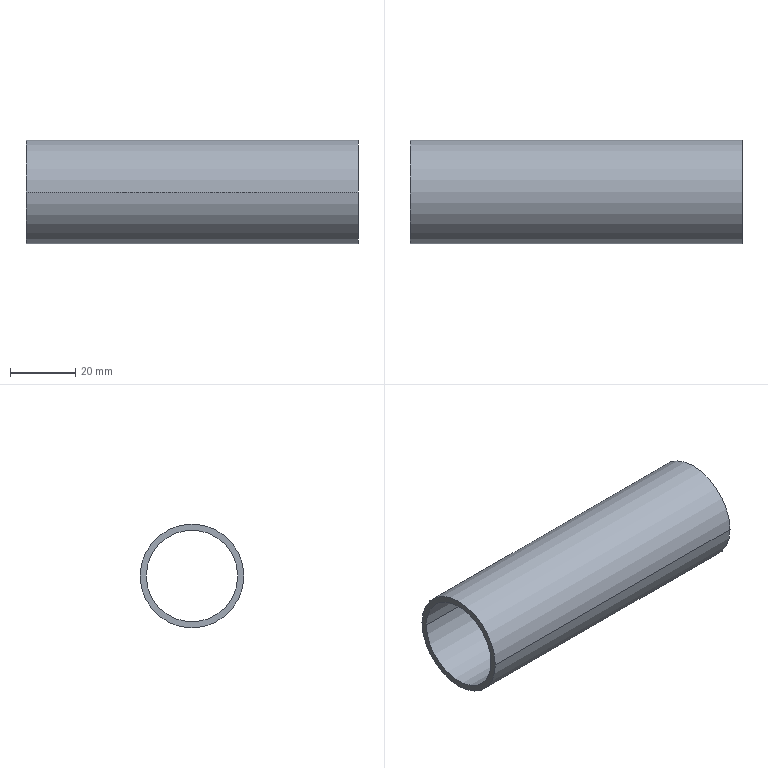Part | NX | features BREP 1 | 1 solid | 6 faces | box 101.6 x 31.75 x 31.75 mm | volume 17920 mm3 | cylinder 4 | plane 2 | commonest cylinder face diameters 27.991 x2 31.75 x2
STEP:
#1=CARTESIAN_POINT('',(0.,15.875,0.));
#2=VERTEX_POINT('',#1);
#3=CARTESIAN_POINT('',(0.,-15.875,0.));
#4=VERTEX_POINT('',#3);
#5=CARTESIAN_POINT('',(0.,0.,0.));
#6=DIRECTION('',(1.,0.,0.));
#7=DIRECTION('',(0.,1.,0.));
#8=AXIS2_PLACEMENT_3D('',#5,#6,#7);
#9=CIRCLE('',#8,15.875);
#10=EDGE_CURVE('',#2,#4,#9,.T.);
#11=ORIENTED_EDGE('',*,*,#10,.F.);
#12=CARTESIAN_POINT('',(0.,0.,0.));
#13=DIRECTION('',(1.,0.,0.));
#14=DIRECTION('',(0.,-1.,0.));
#15=AXIS2_PLACEMENT_3D('',#12,#13,#14);
#16=CIRCLE('',#15,15.875);
#17=EDGE_CURVE('',#4,#2,#16,.T.);
#18=ORIENTED_EDGE('',*,*,#17,.F.);
#19=EDGE_LOOP('',(#11,#18));
#20=FACE_BOUND('',#19,.T.);
#21=CARTESIAN_POINT('',(0.,13.995,0.));
#22=VERTEX_POINT('',#21);
#23=CARTESIAN_POINT('',(0.,-13.995,0.));
#24=VERTEX_POINT('',#23);
#25=CARTESIAN_POINT('',(0.,0.,0.));
#26=DIRECTION('',(-1.,0.,0.));
#27=DIRECTION('',(0.,1.,0.));
#28=AXIS2_PLACEMENT_3D('',#25,#26,#27);
#29=CIRCLE('',#28,13.995);
#30=EDGE_CURVE('',#22,#24,#29,.T.);
#31=ORIENTED_EDGE('',*,*,#30,.F.);
#32=CARTESIAN_POINT('',(0.,0.,0.));
#33=DIRECTION('',(-1.,0.,0.));
#34=DIRECTION('',(0.,-1.,0.));
#35=AXIS2_PLACEMENT_3D('',#32,#33,#34);
#36=CIRCLE('',#35,13.995);
#37=EDGE_CURVE('',#24,#22,#36,.T.);
#38=ORIENTED_EDGE('',*,*,#37,.F.);
#39=EDGE_LOOP('',(#31,#38));
#40=FACE_BOUND('',#39,.T.);
#41=CARTESIAN_POINT('',(0.,0.,0.));
#42=DIRECTION('',(1.,0.,0.));
#43=DIRECTION('',(0.,1.,0.));
#44=AXIS2_PLACEMENT_3D('',#41,#42,#43);
#45=PLANE('',#44);
#46=ADVANCED_FACE('',(#20,#40),#45,.F.);
#47=CARTESIAN_POINT('',(101.6,15.875,0.));
#48=VERTEX_POINT('',#47);
#49=CARTESIAN_POINT('',(0.,15.875,0.));
#50=DIRECTION('',(1.,0.,0.));
#51=VECTOR('',#50,1000.);
#52=LINE('',#49,#51);
#53=EDGE_CURVE('',#48,#2,#52,.F.);
#54=ORIENTED_EDGE('',*,*,#53,.F.);
#55=CARTESIAN_POINT('',(101.6,-15.875,0.));
#56=VERTEX_POINT('',#55);
#57=CARTESIAN_POINT('',(101.6,0.,0.));
#58=DIRECTION('',(1.,0.,0.));
#59=DIRECTION('',(0.,-1.,0.));
#60=AXIS2_PLACEMENT_3D('',#57,#58,#59);
#61=CIRCLE('',#60,15.875);
#62=EDGE_CURVE('',#56,#48,#61,.T.);
#63=ORIENTED_EDGE('',*,*,#62,.F.);
#64=CARTESIAN_POINT('',(0.,-15.875,0.));
#65=DIRECTION('',(1.,0.,0.));
#66=VECTOR('',#65,1000.);
#67=LINE('',#64,#66);
#68=EDGE_CURVE('',#56,#4,#67,.F.);
#69=ORIENTED_EDGE('',*,*,#68,.T.);
#70=ORIENTED_EDGE('',*,*,#17,.T.);
#71=EDGE_LOOP('',(#54,#63,#69,#70));
#72=FACE_BOUND('',#71,.T.);
#73=CARTESIAN_POINT('',(0.,0.,0.));
#74=DIRECTION('',(1.,0.,0.));
#75=DIRECTION('',(0.,-1.,0.));
#76=AXIS2_PLACEMENT_3D('',#73,#74,#75);
#77=CYLINDRICAL_SURFACE('',#76,15.875);
#78=ADVANCED_FACE('',(#72),#77,.T.);
#79=ORIENTED_EDGE('',*,*,#68,.F.);
#80=CARTESIAN_POINT('',(101.6,0.,0.));
#81=DIRECTION('',(1.,0.,0.));
#82=DIRECTION('',(0.,1.,0.));
#83=AXIS2_PLACEMENT_3D('',#80,#81,#82);
#84=CIRCLE('',#83,15.875);
#85=EDGE_CURVE('',#48,#56,#84,.T.);
#86=ORIENTED_EDGE('',*,*,#85,.F.);
#87=ORIENTED_EDGE('',*,*,#53,.T.);
#88=ORIENTED_EDGE('',*,*,#10,.T.);
#89=EDGE_LOOP('',(#79,#86,#87,#88));
#90=FACE_BOUND('',#89,.T.);
#91=CARTESIAN_POINT('',(0.,0.,0.));
#92=DIRECTION('',(1.,0.,0.));
#93=DIRECTION('',(0.,-1.,0.));
#94=AXIS2_PLACEMENT_3D('',#91,#92,#93);
#95=CYLINDRICAL_SURFACE('',#94,15.875);
#96=ADVANCED_FACE('',(#90),#95,.T.);
#97=ORIENTED_EDGE('',*,*,#85,.T.);
#98=ORIENTED_EDGE('',*,*,#62,.T.);
#99=EDGE_LOOP('',(#97,#98));
#100=FACE_BOUND('',#99,.T.);
#101=CARTESIAN_POINT('',(101.6,13.995,0.));
#102=VERTEX_POINT('',#101);
#103=CARTESIAN_POINT('',(101.6,-13.995,0.));
#104=VERTEX_POINT('',#103);
#105=CARTESIAN_POINT('',(101.6,0.,0.));
#106=DIRECTION('',(-1.,0.,0.));
#107=DIRECTION('',(0.,1.,0.));
#108=AXIS2_PLACEMENT_3D('',#105,#106,#107);
#109=CIRCLE('',#108,13.995);
#110=EDGE_CURVE('',#102,#104,#109,.T.);
#111=ORIENTED_EDGE('',*,*,#110,.T.);
#112=CARTESIAN_POINT('',(101.6,0.,0.));
#113=DIRECTION('',(-1.,0.,0.));
#114=DIRECTION('',(0.,-1.,0.));
#115=AXIS2_PLACEMENT_3D('',#112,#113,#114);
#116=CIRCLE('',#115,13.995);
#117=EDGE_CURVE('',#104,#102,#116,.T.);
#118=ORIENTED_EDGE('',*,*,#117,.T.);
#119=EDGE_LOOP('',(#111,#118));
#120=FACE_BOUND('',#119,.T.);
#121=CARTESIAN_POINT('',(101.6,0.,0.));
#122=DIRECTION('',(1.,0.,0.));
#123=DIRECTION('',(0.,1.,0.));
#124=AXIS2_PLACEMENT_3D('',#121,#122,#123);
#125=PLANE('',#124);
#126=ADVANCED_FACE('',(#100,#120),#125,.T.);
#127=CARTESIAN_POINT('',(0.,13.995,0.));
#128=DIRECTION('',(1.,0.,0.));
#129=VECTOR('',#128,1000.);
#130=LINE('',#127,#129);
#131=EDGE_CURVE('',#102,#22,#130,.F.);
#132=ORIENTED_EDGE('',*,*,#131,.F.);
#133=ORIENTED_EDGE('',*,*,#117,.F.);
#134=CARTESIAN_POINT('',(0.,-13.995,0.));
#135=DIRECTION('',(1.,0.,0.));
#136=VECTOR('',#135,1000.);
#137=LINE('',#134,#136);
#138=EDGE_CURVE('',#104,#24,#137,.F.);
#139=ORIENTED_EDGE('',*,*,#138,.T.);
#140=ORIENTED_EDGE('',*,*,#37,.T.);
#141=EDGE_LOOP('',(#132,#133,#139,#140));
#142=FACE_BOUND('',#141,.T.);
#143=CARTESIAN_POINT('',(0.,0.,0.));
#144=DIRECTION('',(1.,0.,0.));
#145=DIRECTION('',(0.,-1.,0.));
#146=AXIS2_PLACEMENT_3D('',#143,#144,#145);
#147=CYLINDRICAL_SURFACE('',#146,13.995);
#148=ADVANCED_FACE('',(#142),#147,.F.);
#149=ORIENTED_EDGE('',*,*,#138,.F.);
#150=ORIENTED_EDGE('',*,*,#110,.F.);
#151=ORIENTED_EDGE('',*,*,#131,.T.);
#152=ORIENTED_EDGE('',*,*,#30,.T.);
#153=EDGE_LOOP('',(#149,#150,#151,#152));
#154=FACE_BOUND('',#153,.T.);
#155=CARTESIAN_POINT('',(0.,0.,0.));
#156=DIRECTION('',(1.,0.,0.));
#157=DIRECTION('',(0.,-1.,0.));
#158=AXIS2_PLACEMENT_3D('',#155,#156,#157);
#159=CYLINDRICAL_SURFACE('',#158,13.995);
#160=ADVANCED_FACE('',(#154),#159,.F.);
#161=CLOSED_SHELL('',(#46,#78,#96,#126,#148,#160));
#162=MANIFOLD_SOLID_BREP('',#161);
#163=(LENGTH_UNIT()NAMED_UNIT(*)SI_UNIT(.MILLI.,.METRE.));
#164=UNCERTAINTY_MEASURE_WITH_UNIT(LENGTH_MEASURE(0.00001),#163,'','');
#165=(NAMED_UNIT(*)PLANE_ANGLE_UNIT()SI_UNIT($,.RADIAN.));
#166=(NAMED_UNIT(*)SI_UNIT($,.STERADIAN.)SOLID_ANGLE_UNIT());
#167=(GEOMETRIC_REPRESENTATION_CONTEXT(3)GLOBAL_UNCERTAINTY_ASSIGNED_CONTEXT((#164))GLOBAL_UNIT_ASSIGNED_CONTEXT((#163,#165,#166))REPRESENTATION_CONTEXT('',''));
#168=ADVANCED_BREP_SHAPE_REPRESENTATION('',(#162),#167);